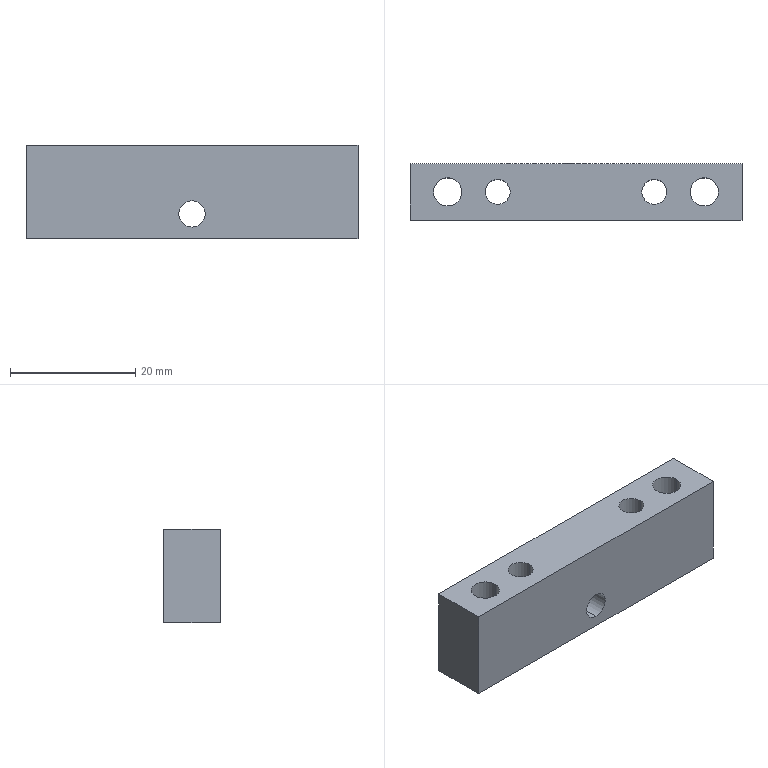Part | STEP file | 11-FG-B02411 | 1 solid | 22 faces | box 53 x 9 x 15 mm | volume 5874 mm3 | cylinder 14 | plane 8 | commonest cylinder face diameters 4 x4 4.5 x4 8 x4 4.2 x2
STEP:
#1=CARTESIAN_POINT('',(41.,4.5,15.));
#2=VERTEX_POINT('',#1);
#3=CARTESIAN_POINT('',(37.,4.5,15.));
#4=VERTEX_POINT('',#3);
#5=CARTESIAN_POINT('',(39.,4.5,15.));
#6=DIRECTION('',(0.,0.,-1.));
#7=DIRECTION('',(-1.,0.,0.));
#8=AXIS2_PLACEMENT_3D('',#5,#6,#7);
#9=CIRCLE('',#8,2.);
#10=EDGE_CURVE('',#2,#4,#9,.T.);
#11=ORIENTED_EDGE('',*,*,#10,.F.);
#12=CARTESIAN_POINT('',(41.,4.5,0.));
#13=VERTEX_POINT('',#12);
#14=CARTESIAN_POINT('',(41.,4.5,0.));
#15=DIRECTION('',(0.,0.,-1.));
#16=VECTOR('',#15,1000.);
#17=LINE('',#14,#16);
#18=EDGE_CURVE('',#2,#13,#17,.T.);
#19=ORIENTED_EDGE('',*,*,#18,.T.);
#20=CARTESIAN_POINT('',(37.,4.5,0.));
#21=VERTEX_POINT('',#20);
#22=CARTESIAN_POINT('',(39.,4.5,0.));
#23=DIRECTION('',(0.,0.,-1.));
#24=DIRECTION('',(-1.,0.,0.));
#25=AXIS2_PLACEMENT_3D('',#22,#23,#24);
#26=CIRCLE('',#25,2.);
#27=EDGE_CURVE('',#13,#21,#26,.T.);
#28=ORIENTED_EDGE('',*,*,#27,.T.);
#29=CARTESIAN_POINT('',(37.,4.5,0.));
#30=DIRECTION('',(0.,0.,-1.));
#31=VECTOR('',#30,1000.);
#32=LINE('',#29,#31);
#33=EDGE_CURVE('',#4,#21,#32,.T.);
#34=ORIENTED_EDGE('',*,*,#33,.F.);
#35=EDGE_LOOP('',(#11,#19,#28,#34));
#36=FACE_OUTER_BOUND('',#35,.T.);
#37=CARTESIAN_POINT('',(39.,4.5,0.));
#38=DIRECTION('',(0.,0.,-1.));
#39=DIRECTION('',(-1.,0.,0.));
#40=AXIS2_PLACEMENT_3D('',#37,#38,#39);
#41=CYLINDRICAL_SURFACE('',#40,2.);
#42=ADVANCED_FACE('',(#36),#41,.F.);
#43=CARTESIAN_POINT('',(16.,4.5,15.));
#44=VERTEX_POINT('',#43);
#45=CARTESIAN_POINT('',(12.,4.5,15.));
#46=VERTEX_POINT('',#45);
#47=CARTESIAN_POINT('',(14.,4.5,15.));
#48=DIRECTION('',(0.,0.,-1.));
#49=DIRECTION('',(-1.,0.,0.));
#50=AXIS2_PLACEMENT_3D('',#47,#48,#49);
#51=CIRCLE('',#50,2.);
#52=EDGE_CURVE('',#44,#46,#51,.T.);
#53=ORIENTED_EDGE('',*,*,#52,.F.);
#54=CARTESIAN_POINT('',(16.,4.5,0.));
#55=VERTEX_POINT('',#54);
#56=CARTESIAN_POINT('',(16.,4.5,0.));
#57=DIRECTION('',(0.,0.,-1.));
#58=VECTOR('',#57,1000.);
#59=LINE('',#56,#58);
#60=EDGE_CURVE('',#44,#55,#59,.T.);
#61=ORIENTED_EDGE('',*,*,#60,.T.);
#62=CARTESIAN_POINT('',(12.,4.5,0.));
#63=VERTEX_POINT('',#62);
#64=CARTESIAN_POINT('',(14.,4.5,0.));
#65=DIRECTION('',(0.,0.,-1.));
#66=DIRECTION('',(-1.,0.,0.));
#67=AXIS2_PLACEMENT_3D('',#64,#65,#66);
#68=CIRCLE('',#67,2.);
#69=EDGE_CURVE('',#55,#63,#68,.T.);
#70=ORIENTED_EDGE('',*,*,#69,.T.);
#71=CARTESIAN_POINT('',(12.,4.5,0.));
#72=DIRECTION('',(0.,0.,-1.));
#73=VECTOR('',#72,1000.);
#74=LINE('',#71,#73);
#75=EDGE_CURVE('',#46,#63,#74,.T.);
#76=ORIENTED_EDGE('',*,*,#75,.F.);
#77=EDGE_LOOP('',(#53,#61,#70,#76));
#78=FACE_OUTER_BOUND('',#77,.T.);
#79=CARTESIAN_POINT('',(14.,4.5,0.));
#80=DIRECTION('',(0.,0.,-1.));
#81=DIRECTION('',(-1.,0.,0.));
#82=AXIS2_PLACEMENT_3D('',#79,#80,#81);
#83=CYLINDRICAL_SURFACE('',#82,2.);
#84=ADVANCED_FACE('',(#78),#83,.F.);
#85=CARTESIAN_POINT('',(26.5,0.,1.9));
#86=VERTEX_POINT('',#85);
#87=CARTESIAN_POINT('',(26.5,0.,6.1));
#88=VERTEX_POINT('',#87);
#89=CARTESIAN_POINT('',(26.5,0.,4.));
#90=DIRECTION('',(0.,1.,0.));
#91=DIRECTION('',(0.,0.,1.));
#92=AXIS2_PLACEMENT_3D('',#89,#90,#91);
#93=CIRCLE('',#92,2.1);
#94=EDGE_CURVE('',#86,#88,#93,.T.);
#95=ORIENTED_EDGE('',*,*,#94,.F.);
#96=CARTESIAN_POINT('',(26.5,9.,1.9));
#97=VERTEX_POINT('',#96);
#98=CARTESIAN_POINT('',(26.5,9.,1.9));
#99=DIRECTION('',(0.,1.,0.));
#100=VECTOR('',#99,1000.);
#101=LINE('',#98,#100);
#102=EDGE_CURVE('',#86,#97,#101,.T.);
#103=ORIENTED_EDGE('',*,*,#102,.T.);
#104=CARTESIAN_POINT('',(26.5,9.,6.1));
#105=VERTEX_POINT('',#104);
#106=CARTESIAN_POINT('',(26.5,9.,4.));
#107=DIRECTION('',(0.,1.,0.));
#108=DIRECTION('',(0.,0.,1.));
#109=AXIS2_PLACEMENT_3D('',#106,#107,#108);
#110=CIRCLE('',#109,2.1);
#111=EDGE_CURVE('',#97,#105,#110,.T.);
#112=ORIENTED_EDGE('',*,*,#111,.T.);
#113=CARTESIAN_POINT('',(26.5,9.,6.1));
#114=DIRECTION('',(0.,1.,0.));
#115=VECTOR('',#114,1000.);
#116=LINE('',#113,#115);
#117=EDGE_CURVE('',#88,#105,#116,.T.);
#118=ORIENTED_EDGE('',*,*,#117,.F.);
#119=EDGE_LOOP('',(#95,#103,#112,#118));
#120=FACE_OUTER_BOUND('',#119,.T.);
#121=CARTESIAN_POINT('',(26.5,9.,4.));
#122=DIRECTION('',(0.,1.,0.));
#123=DIRECTION('',(0.,0.,1.));
#124=AXIS2_PLACEMENT_3D('',#121,#122,#123);
#125=CYLINDRICAL_SURFACE('',#124,2.1);
#126=ADVANCED_FACE('',(#120),#125,.F.);
#127=CARTESIAN_POINT('',(51.,4.5,4.4));
#128=VERTEX_POINT('',#127);
#129=CARTESIAN_POINT('',(43.,4.5,4.4));
#130=VERTEX_POINT('',#129);
#131=CARTESIAN_POINT('',(47.,4.5,4.4));
#132=DIRECTION('',(0.,0.,-1.));
#133=DIRECTION('',(-1.,0.,0.));
#134=AXIS2_PLACEMENT_3D('',#131,#132,#133);
#135=CIRCLE('',#134,4.);
#136=EDGE_CURVE('',#128,#130,#135,.T.);
#137=ORIENTED_EDGE('',*,*,#136,.F.);
#138=CARTESIAN_POINT('',(51.,4.5,0.));
#139=VERTEX_POINT('',#138);
#140=CARTESIAN_POINT('',(51.,4.5,0.));
#141=DIRECTION('',(0.,0.,-1.));
#142=VECTOR('',#141,1000.);
#143=LINE('',#140,#142);
#144=EDGE_CURVE('',#128,#139,#143,.T.);
#145=ORIENTED_EDGE('',*,*,#144,.T.);
#146=CARTESIAN_POINT('',(43.,4.5,0.));
#147=VERTEX_POINT('',#146);
#148=CARTESIAN_POINT('',(47.,4.5,0.));
#149=DIRECTION('',(0.,0.,-1.));
#150=DIRECTION('',(-1.,0.,0.));
#151=AXIS2_PLACEMENT_3D('',#148,#149,#150);
#152=CIRCLE('',#151,4.);
#153=EDGE_CURVE('',#139,#147,#152,.T.);
#154=ORIENTED_EDGE('',*,*,#153,.T.);
#155=CARTESIAN_POINT('',(43.,4.5,0.));
#156=DIRECTION('',(0.,0.,-1.));
#157=VECTOR('',#156,1000.);
#158=LINE('',#155,#157);
#159=EDGE_CURVE('',#130,#147,#158,.T.);
#160=ORIENTED_EDGE('',*,*,#159,.F.);
#161=EDGE_LOOP('',(#137,#145,#154,#160));
#162=FACE_OUTER_BOUND('',#161,.T.);
#163=CARTESIAN_POINT('',(47.,4.5,0.));
#164=DIRECTION('',(0.,0.,-1.));
#165=DIRECTION('',(-1.,0.,0.));
#166=AXIS2_PLACEMENT_3D('',#163,#164,#165);
#167=CYLINDRICAL_SURFACE('',#166,4.);
#168=ADVANCED_FACE('',(#162),#167,.F.);
#169=CARTESIAN_POINT('',(49.25,4.5,15.));
#170=VERTEX_POINT('',#169);
#171=CARTESIAN_POINT('',(44.75,4.5,15.));
#172=VERTEX_POINT('',#171);
#173=CARTESIAN_POINT('',(47.,4.5,15.));
#174=DIRECTION('',(0.,0.,-1.));
#175=DIRECTION('',(-1.,0.,0.));
#176=AXIS2_PLACEMENT_3D('',#173,#174,#175);
#177=CIRCLE('',#176,2.25);
#178=EDGE_CURVE('',#170,#172,#177,.T.);
#179=ORIENTED_EDGE('',*,*,#178,.F.);
#180=CARTESIAN_POINT('',(49.25,4.5,4.4));
#181=VERTEX_POINT('',#180);
#182=CARTESIAN_POINT('',(49.25,4.5,0.));
#183=DIRECTION('',(0.,0.,-1.));
#184=VECTOR('',#183,1000.);
#185=LINE('',#182,#184);
#186=EDGE_CURVE('',#170,#181,#185,.T.);
#187=ORIENTED_EDGE('',*,*,#186,.T.);
#188=CARTESIAN_POINT('',(44.75,4.5,4.4));
#189=VERTEX_POINT('',#188);
#190=CARTESIAN_POINT('',(47.,4.5,4.4));
#191=DIRECTION('',(0.,0.,-1.));
#192=DIRECTION('',(-1.,0.,0.));
#193=AXIS2_PLACEMENT_3D('',#190,#191,#192);
#194=CIRCLE('',#193,2.25);
#195=EDGE_CURVE('',#181,#189,#194,.T.);
#196=ORIENTED_EDGE('',*,*,#195,.T.);
#197=CARTESIAN_POINT('',(44.75,4.5,0.));
#198=DIRECTION('',(0.,0.,-1.));
#199=VECTOR('',#198,1000.);
#200=LINE('',#197,#199);
#201=EDGE_CURVE('',#172,#189,#200,.T.);
#202=ORIENTED_EDGE('',*,*,#201,.F.);
#203=EDGE_LOOP('',(#179,#187,#196,#202));
#204=FACE_OUTER_BOUND('',#203,.T.);
#205=CARTESIAN_POINT('',(47.,4.5,0.));
#206=DIRECTION('',(0.,0.,-1.));
#207=DIRECTION('',(-1.,0.,0.));
#208=AXIS2_PLACEMENT_3D('',#205,#206,#207);
#209=CYLINDRICAL_SURFACE('',#208,2.25);
#210=ADVANCED_FACE('',(#204),#209,.F.);
#211=CARTESIAN_POINT('',(10.,4.5,4.4));
#212=VERTEX_POINT('',#211);
#213=CARTESIAN_POINT('',(2.,4.5,4.4));
#214=VERTEX_POINT('',#213);
#215=CARTESIAN_POINT('',(6.,4.5,4.4));
#216=DIRECTION('',(0.,0.,-1.));
#217=DIRECTION('',(-1.,0.,0.));
#218=AXIS2_PLACEMENT_3D('',#215,#216,#217);
#219=CIRCLE('',#218,4.);
#220=EDGE_CURVE('',#212,#214,#219,.T.);
#221=ORIENTED_EDGE('',*,*,#220,.F.);
#222=CARTESIAN_POINT('',(10.,4.5,0.));
#223=VERTEX_POINT('',#222);
#224=CARTESIAN_POINT('',(10.,4.5,0.));
#225=DIRECTION('',(0.,0.,-1.));
#226=VECTOR('',#225,1000.);
#227=LINE('',#224,#226);
#228=EDGE_CURVE('',#212,#223,#227,.T.);
#229=ORIENTED_EDGE('',*,*,#228,.T.);
#230=CARTESIAN_POINT('',(2.,4.5,0.));
#231=VERTEX_POINT('',#230);
#232=CARTESIAN_POINT('',(6.,4.5,0.));
#233=DIRECTION('',(0.,0.,-1.));
#234=DIRECTION('',(-1.,0.,0.));
#235=AXIS2_PLACEMENT_3D('',#232,#233,#234);
#236=CIRCLE('',#235,4.);
#237=EDGE_CURVE('',#223,#231,#236,.T.);
#238=ORIENTED_EDGE('',*,*,#237,.T.);
#239=CARTESIAN_POINT('',(2.,4.5,0.));
#240=DIRECTION('',(0.,0.,-1.));
#241=VECTOR('',#240,1000.);
#242=LINE('',#239,#241);
#243=EDGE_CURVE('',#214,#231,#242,.T.);
#244=ORIENTED_EDGE('',*,*,#243,.F.);
#245=EDGE_LOOP('',(#221,#229,#238,#244));
#246=FACE_OUTER_BOUND('',#245,.T.);
#247=CARTESIAN_POINT('',(6.,4.5,0.));
#248=DIRECTION('',(0.,0.,-1.));
#249=DIRECTION('',(-1.,0.,0.));
#250=AXIS2_PLACEMENT_3D('',#247,#248,#249);
#251=CYLINDRICAL_SURFACE('',#250,4.);
#252=ADVANCED_FACE('',(#246),#251,.F.);
#253=CARTESIAN_POINT('',(8.25,4.5,15.));
#254=VERTEX_POINT('',#253);
#255=CARTESIAN_POINT('',(3.75,4.5,15.));
#256=VERTEX_POINT('',#255);
#257=CARTESIAN_POINT('',(6.,4.5,15.));
#258=DIRECTION('',(0.,0.,-1.));
#259=DIRECTION('',(-1.,0.,0.));
#260=AXIS2_PLACEMENT_3D('',#257,#258,#259);
#261=CIRCLE('',#260,2.25);
#262=EDGE_CURVE('',#254,#256,#261,.T.);
#263=ORIENTED_EDGE('',*,*,#262,.F.);
#264=CARTESIAN_POINT('',(8.25,4.5,4.4));
#265=VERTEX_POINT('',#264);
#266=CARTESIAN_POINT('',(8.25,4.5,0.));
#267=DIRECTION('',(0.,0.,-1.));
#268=VECTOR('',#267,1000.);
#269=LINE('',#266,#268);
#270=EDGE_CURVE('',#254,#265,#269,.T.);
#271=ORIENTED_EDGE('',*,*,#270,.T.);
#272=CARTESIAN_POINT('',(3.75,4.5,4.4));
#273=VERTEX_POINT('',#272);
#274=CARTESIAN_POINT('',(6.,4.5,4.4));
#275=DIRECTION('',(0.,0.,-1.));
#276=DIRECTION('',(-1.,0.,0.));
#277=AXIS2_PLACEMENT_3D('',#274,#275,#276);
#278=CIRCLE('',#277,2.25);
#279=EDGE_CURVE('',#265,#273,#278,.T.);
#280=ORIENTED_EDGE('',*,*,#279,.T.);
#281=CARTESIAN_POINT('',(3.75,4.5,0.));
#282=DIRECTION('',(0.,0.,-1.));
#283=VECTOR('',#282,1000.);
#284=LINE('',#281,#283);
#285=EDGE_CURVE('',#256,#273,#284,.T.);
#286=ORIENTED_EDGE('',*,*,#285,.F.);
#287=EDGE_LOOP('',(#263,#271,#280,#286));
#288=FACE_OUTER_BOUND('',#287,.T.);
#289=CARTESIAN_POINT('',(6.,4.5,0.));
#290=DIRECTION('',(0.,0.,-1.));
#291=DIRECTION('',(-1.,0.,0.));
#292=AXIS2_PLACEMENT_3D('',#289,#290,#291);
#293=CYLINDRICAL_SURFACE('',#292,2.25);
#294=ADVANCED_FACE('',(#288),#293,.F.);
#295=CARTESIAN_POINT('',(0.,9.,0.));
#296=VERTEX_POINT('',#295);
#297=CARTESIAN_POINT('',(0.,0.,0.));
#298=VERTEX_POINT('',#297);
#299=CARTESIAN_POINT('',(0.,0.,0.));
#300=DIRECTION('',(0.,-1.,0.));
#301=VECTOR('',#300,1000.);
#302=LINE('',#299,#301);
#303=EDGE_CURVE('',#296,#298,#302,.T.);
#304=ORIENTED_EDGE('',*,*,#303,.T.);
#305=CARTESIAN_POINT('',(0.,0.,15.));
#306=VERTEX_POINT('',#305);
#307=CARTESIAN_POINT('',(0.,0.,15.));
#308=DIRECTION('',(0.,0.,-1.));
#309=VECTOR('',#308,1000.);
#310=LINE('',#307,#309);
#311=EDGE_CURVE('',#306,#298,#310,.T.);
#312=ORIENTED_EDGE('',*,*,#311,.F.);
#313=CARTESIAN_POINT('',(0.,9.,15.));
#314=VERTEX_POINT('',#313);
#315=CARTESIAN_POINT('',(0.,0.,15.));
#316=DIRECTION('',(0.,-1.,0.));
#317=VECTOR('',#316,1000.);
#318=LINE('',#315,#317);
#319=EDGE_CURVE('',#314,#306,#318,.T.);
#320=ORIENTED_EDGE('',*,*,#319,.F.);
#321=CARTESIAN_POINT('',(0.,9.,15.));
#322=DIRECTION('',(0.,0.,-1.));
#323=VECTOR('',#322,1000.);
#324=LINE('',#321,#323);
#325=EDGE_CURVE('',#314,#296,#324,.T.);
#326=ORIENTED_EDGE('',*,*,#325,.T.);
#327=EDGE_LOOP('',(#304,#312,#320,#326));
#328=FACE_OUTER_BOUND('',#327,.T.);
#329=CARTESIAN_POINT('',(0.,0.,15.));
#330=DIRECTION('',(1.,0.,0.));
#331=DIRECTION('',(0.,1.,0.));
#332=AXIS2_PLACEMENT_3D('',#329,#330,#331);
#333=PLANE('',#332);
#334=ADVANCED_FACE('',(#328),#333,.F.);
#335=CARTESIAN_POINT('',(26.5,0.,4.));
#336=DIRECTION('',(0.,1.,0.));
#337=DIRECTION('',(0.,0.,1.));
#338=AXIS2_PLACEMENT_3D('',#335,#336,#337);
#339=CIRCLE('',#338,2.1);
#340=EDGE_CURVE('',#88,#86,#339,.T.);
#341=ORIENTED_EDGE('',*,*,#340,.T.);
#342=ORIENTED_EDGE('',*,*,#94,.T.);
#343=EDGE_LOOP('',(#341,#342));
#344=FACE_BOUND('',#343,.T.);
#345=CARTESIAN_POINT('',(53.,0.,0.));
#346=VERTEX_POINT('',#345);
#347=CARTESIAN_POINT('',(0.,0.,0.));
#348=DIRECTION('',(1.,0.,0.));
#349=VECTOR('',#348,1000.);
#350=LINE('',#347,#349);
#351=EDGE_CURVE('',#298,#346,#350,.T.);
#352=ORIENTED_EDGE('',*,*,#351,.T.);
#353=CARTESIAN_POINT('',(53.,0.,15.));
#354=VERTEX_POINT('',#353);
#355=CARTESIAN_POINT('',(53.,0.,15.));
#356=DIRECTION('',(0.,0.,-1.));
#357=VECTOR('',#356,1000.);
#358=LINE('',#355,#357);
#359=EDGE_CURVE('',#354,#346,#358,.T.);
#360=ORIENTED_EDGE('',*,*,#359,.F.);
#361=CARTESIAN_POINT('',(0.,0.,15.));
#362=DIRECTION('',(1.,0.,0.));
#363=VECTOR('',#362,1000.);
#364=LINE('',#361,#363);
#365=EDGE_CURVE('',#306,#354,#364,.T.);
#366=ORIENTED_EDGE('',*,*,#365,.F.);
#367=ORIENTED_EDGE('',*,*,#311,.T.);
#368=EDGE_LOOP('',(#352,#360,#366,#367));
#369=FACE_OUTER_BOUND('',#368,.T.);
#370=CARTESIAN_POINT('',(0.,0.,15.));
#371=DIRECTION('',(0.,1.,0.));
#372=DIRECTION('',(0.,0.,1.));
#373=AXIS2_PLACEMENT_3D('',#370,#371,#372);
#374=PLANE('',#373);
#375=ADVANCED_FACE('',(#344,#369),#374,.F.);
#376=CARTESIAN_POINT('',(53.,9.,0.));
#377=VERTEX_POINT('',#376);
#378=CARTESIAN_POINT('',(53.,0.,0.));
#379=DIRECTION('',(0.,1.,0.));
#380=VECTOR('',#379,1000.);
#381=LINE('',#378,#380);
#382=EDGE_CURVE('',#346,#377,#381,.T.);
#383=ORIENTED_EDGE('',*,*,#382,.T.);
#384=CARTESIAN_POINT('',(53.,9.,15.));
#385=VERTEX_POINT('',#384);
#386=CARTESIAN_POINT('',(53.,9.,15.));
#387=DIRECTION('',(0.,0.,-1.));
#388=VECTOR('',#387,1000.);
#389=LINE('',#386,#388);
#390=EDGE_CURVE('',#385,#377,#389,.T.);
#391=ORIENTED_EDGE('',*,*,#390,.F.);
#392=CARTESIAN_POINT('',(53.,0.,15.));
#393=DIRECTION('',(0.,1.,0.));
#394=VECTOR('',#393,1000.);
#395=LINE('',#392,#394);
#396=EDGE_CURVE('',#354,#385,#395,.T.);
#397=ORIENTED_EDGE('',*,*,#396,.F.);
#398=ORIENTED_EDGE('',*,*,#359,.T.);
#399=EDGE_LOOP('',(#383,#391,#397,#398));
#400=FACE_OUTER_BOUND('',#399,.T.);
#401=CARTESIAN_POINT('',(53.,0.,15.));
#402=DIRECTION('',(-1.,0.,0.));
#403=DIRECTION('',(0.,-1.,0.));
#404=AXIS2_PLACEMENT_3D('',#401,#402,#403);
#405=PLANE('',#404);
#406=ADVANCED_FACE('',(#400),#405,.F.);
#407=CARTESIAN_POINT('',(26.5,9.,4.));
#408=DIRECTION('',(0.,1.,0.));
#409=DIRECTION('',(0.,0.,1.));
#410=AXIS2_PLACEMENT_3D('',#407,#408,#409);
#411=CIRCLE('',#410,2.1);
#412=EDGE_CURVE('',#105,#97,#411,.T.);
#413=ORIENTED_EDGE('',*,*,#412,.F.);
#414=ORIENTED_EDGE('',*,*,#111,.F.);
#415=EDGE_LOOP('',(#413,#414));
#416=FACE_BOUND('',#415,.T.);
#417=CARTESIAN_POINT('',(0.,9.,0.));
#418=DIRECTION('',(-1.,0.,0.));
#419=VECTOR('',#418,1000.);
#420=LINE('',#417,#419);
#421=EDGE_CURVE('',#377,#296,#420,.T.);
#422=ORIENTED_EDGE('',*,*,#421,.T.);
#423=ORIENTED_EDGE('',*,*,#325,.F.);
#424=CARTESIAN_POINT('',(0.,9.,15.));
#425=DIRECTION('',(-1.,0.,0.));
#426=VECTOR('',#425,1000.);
#427=LINE('',#424,#426);
#428=EDGE_CURVE('',#385,#314,#427,.T.);
#429=ORIENTED_EDGE('',*,*,#428,.F.);
#430=ORIENTED_EDGE('',*,*,#390,.T.);
#431=EDGE_LOOP('',(#422,#423,#429,#430));
#432=FACE_OUTER_BOUND('',#431,.T.);
#433=CARTESIAN_POINT('',(0.,9.,15.));
#434=DIRECTION('',(0.,-1.,0.));
#435=DIRECTION('',(0.,0.,-1.));
#436=AXIS2_PLACEMENT_3D('',#433,#434,#435);
#437=PLANE('',#436);
#438=ADVANCED_FACE('',(#416,#432),#437,.F.);
#439=CARTESIAN_POINT('',(39.,4.5,15.));
#440=DIRECTION('',(0.,0.,-1.));
#441=DIRECTION('',(-1.,0.,0.));
#442=AXIS2_PLACEMENT_3D('',#439,#440,#441);
#443=CIRCLE('',#442,2.);
#444=EDGE_CURVE('',#4,#2,#443,.T.);
#445=ORIENTED_EDGE('',*,*,#444,.T.);
#446=ORIENTED_EDGE('',*,*,#10,.T.);
#447=EDGE_LOOP('',(#445,#446));
#448=FACE_BOUND('',#447,.T.);
#449=CARTESIAN_POINT('',(14.,4.5,15.));
#450=DIRECTION('',(0.,0.,-1.));
#451=DIRECTION('',(-1.,0.,0.));
#452=AXIS2_PLACEMENT_3D('',#449,#450,#451);
#453=CIRCLE('',#452,2.);
#454=EDGE_CURVE('',#46,#44,#453,.T.);
#455=ORIENTED_EDGE('',*,*,#454,.T.);
#456=ORIENTED_EDGE('',*,*,#52,.T.);
#457=EDGE_LOOP('',(#455,#456));
#458=FACE_BOUND('',#457,.T.);
#459=CARTESIAN_POINT('',(47.,4.5,15.));
#460=DIRECTION('',(0.,0.,-1.));
#461=DIRECTION('',(-1.,0.,0.));
#462=AXIS2_PLACEMENT_3D('',#459,#460,#461);
#463=CIRCLE('',#462,2.25);
#464=EDGE_CURVE('',#172,#170,#463,.T.);
#465=ORIENTED_EDGE('',*,*,#464,.T.);
#466=ORIENTED_EDGE('',*,*,#178,.T.);
#467=EDGE_LOOP('',(#465,#466));
#468=FACE_BOUND('',#467,.T.);
#469=CARTESIAN_POINT('',(6.,4.5,15.));
#470=DIRECTION('',(0.,0.,-1.));
#471=DIRECTION('',(-1.,0.,0.));
#472=AXIS2_PLACEMENT_3D('',#469,#470,#471);
#473=CIRCLE('',#472,2.25);
#474=EDGE_CURVE('',#256,#254,#473,.T.);
#475=ORIENTED_EDGE('',*,*,#474,.T.);
#476=ORIENTED_EDGE('',*,*,#262,.T.);
#477=EDGE_LOOP('',(#475,#476));
#478=FACE_BOUND('',#477,.T.);
#479=ORIENTED_EDGE('',*,*,#319,.T.);
#480=ORIENTED_EDGE('',*,*,#365,.T.);
#481=ORIENTED_EDGE('',*,*,#396,.T.);
#482=ORIENTED_EDGE('',*,*,#428,.T.);
#483=EDGE_LOOP('',(#479,#480,#481,#482));
#484=FACE_OUTER_BOUND('',#483,.T.);
#485=CARTESIAN_POINT('',(0.,9.,15.));
#486=DIRECTION('',(0.,0.,-1.));
#487=DIRECTION('',(-1.,0.,0.));
#488=AXIS2_PLACEMENT_3D('',#485,#486,#487);
#489=PLANE('',#488);
#490=ADVANCED_FACE('',(#448,#458,#468,#478,#484),#489,.F.);
#491=CARTESIAN_POINT('',(39.,4.5,0.));
#492=DIRECTION('',(0.,0.,-1.));
#493=DIRECTION('',(-1.,0.,0.));
#494=AXIS2_PLACEMENT_3D('',#491,#492,#493);
#495=CIRCLE('',#494,2.);
#496=EDGE_CURVE('',#21,#13,#495,.T.);
#497=ORIENTED_EDGE('',*,*,#496,.F.);
#498=ORIENTED_EDGE('',*,*,#27,.F.);
#499=EDGE_LOOP('',(#497,#498));
#500=FACE_BOUND('',#499,.T.);
#501=CARTESIAN_POINT('',(14.,4.5,0.));
#502=DIRECTION('',(0.,0.,-1.));
#503=DIRECTION('',(-1.,0.,0.));
#504=AXIS2_PLACEMENT_3D('',#501,#502,#503);
#505=CIRCLE('',#504,2.);
#506=EDGE_CURVE('',#63,#55,#505,.T.);
#507=ORIENTED_EDGE('',*,*,#506,.F.);
#508=ORIENTED_EDGE('',*,*,#69,.F.);
#509=EDGE_LOOP('',(#507,#508));
#510=FACE_BOUND('',#509,.T.);
#511=CARTESIAN_POINT('',(47.,4.5,0.));
#512=DIRECTION('',(0.,0.,-1.));
#513=DIRECTION('',(-1.,0.,0.));
#514=AXIS2_PLACEMENT_3D('',#511,#512,#513);
#515=CIRCLE('',#514,4.);
#516=EDGE_CURVE('',#147,#139,#515,.T.);
#517=ORIENTED_EDGE('',*,*,#516,.F.);
#518=ORIENTED_EDGE('',*,*,#153,.F.);
#519=EDGE_LOOP('',(#517,#518));
#520=FACE_BOUND('',#519,.T.);
#521=CARTESIAN_POINT('',(6.,4.5,0.));
#522=DIRECTION('',(0.,0.,-1.));
#523=DIRECTION('',(-1.,0.,0.));
#524=AXIS2_PLACEMENT_3D('',#521,#522,#523);
#525=CIRCLE('',#524,4.);
#526=EDGE_CURVE('',#231,#223,#525,.T.);
#527=ORIENTED_EDGE('',*,*,#526,.F.);
#528=ORIENTED_EDGE('',*,*,#237,.F.);
#529=EDGE_LOOP('',(#527,#528));
#530=FACE_BOUND('',#529,.T.);
#531=ORIENTED_EDGE('',*,*,#303,.F.);
#532=ORIENTED_EDGE('',*,*,#421,.F.);
#533=ORIENTED_EDGE('',*,*,#382,.F.);
#534=ORIENTED_EDGE('',*,*,#351,.F.);
#535=EDGE_LOOP('',(#531,#532,#533,#534));
#536=FACE_OUTER_BOUND('',#535,.T.);
#537=CARTESIAN_POINT('',(0.,9.,0.));
#538=DIRECTION('',(0.,0.,-1.));
#539=DIRECTION('',(-1.,0.,0.));
#540=AXIS2_PLACEMENT_3D('',#537,#538,#539);
#541=PLANE('',#540);
#542=ADVANCED_FACE('',(#500,#510,#520,#530,#536),#541,.T.);
#543=ORIENTED_EDGE('',*,*,#270,.F.);
#544=ORIENTED_EDGE('',*,*,#474,.F.);
#545=ORIENTED_EDGE('',*,*,#285,.T.);
#546=CARTESIAN_POINT('',(6.,4.5,4.4));
#547=DIRECTION('',(0.,0.,-1.));
#548=DIRECTION('',(-1.,0.,0.));
#549=AXIS2_PLACEMENT_3D('',#546,#547,#548);
#550=CIRCLE('',#549,2.25);
#551=EDGE_CURVE('',#273,#265,#550,.T.);
#552=ORIENTED_EDGE('',*,*,#551,.T.);
#553=EDGE_LOOP('',(#543,#544,#545,#552));
#554=FACE_OUTER_BOUND('',#553,.T.);
#555=CARTESIAN_POINT('',(6.,4.5,0.));
#556=DIRECTION('',(0.,0.,-1.));
#557=DIRECTION('',(-1.,0.,0.));
#558=AXIS2_PLACEMENT_3D('',#555,#556,#557);
#559=CYLINDRICAL_SURFACE('',#558,2.25);
#560=ADVANCED_FACE('',(#554),#559,.F.);
#561=ORIENTED_EDGE('',*,*,#551,.F.);
#562=ORIENTED_EDGE('',*,*,#279,.F.);
#563=EDGE_LOOP('',(#561,#562));
#564=FACE_BOUND('',#563,.T.);
#565=CARTESIAN_POINT('',(6.,4.5,4.4));
#566=DIRECTION('',(0.,0.,-1.));
#567=DIRECTION('',(-1.,0.,0.));
#568=AXIS2_PLACEMENT_3D('',#565,#566,#567);
#569=CIRCLE('',#568,4.);
#570=EDGE_CURVE('',#214,#212,#569,.T.);
#571=ORIENTED_EDGE('',*,*,#570,.T.);
#572=ORIENTED_EDGE('',*,*,#220,.T.);
#573=EDGE_LOOP('',(#571,#572));
#574=FACE_OUTER_BOUND('',#573,.T.);
#575=CARTESIAN_POINT('',(8.25,4.5,4.4));
#576=DIRECTION('',(0.,0.,1.));
#577=DIRECTION('',(1.,0.,0.));
#578=AXIS2_PLACEMENT_3D('',#575,#576,#577);
#579=PLANE('',#578);
#580=ADVANCED_FACE('',(#564,#574),#579,.F.);
#581=ORIENTED_EDGE('',*,*,#228,.F.);
#582=ORIENTED_EDGE('',*,*,#570,.F.);
#583=ORIENTED_EDGE('',*,*,#243,.T.);
#584=ORIENTED_EDGE('',*,*,#526,.T.);
#585=EDGE_LOOP('',(#581,#582,#583,#584));
#586=FACE_OUTER_BOUND('',#585,.T.);
#587=CARTESIAN_POINT('',(6.,4.5,0.));
#588=DIRECTION('',(0.,0.,-1.));
#589=DIRECTION('',(-1.,0.,0.));
#590=AXIS2_PLACEMENT_3D('',#587,#588,#589);
#591=CYLINDRICAL_SURFACE('',#590,4.);
#592=ADVANCED_FACE('',(#586),#591,.F.);
#593=ORIENTED_EDGE('',*,*,#186,.F.);
#594=ORIENTED_EDGE('',*,*,#464,.F.);
#595=ORIENTED_EDGE('',*,*,#201,.T.);
#596=CARTESIAN_POINT('',(47.,4.5,4.4));
#597=DIRECTION('',(0.,0.,-1.));
#598=DIRECTION('',(-1.,0.,0.));
#599=AXIS2_PLACEMENT_3D('',#596,#597,#598);
#600=CIRCLE('',#599,2.25);
#601=EDGE_CURVE('',#189,#181,#600,.T.);
#602=ORIENTED_EDGE('',*,*,#601,.T.);
#603=EDGE_LOOP('',(#593,#594,#595,#602));
#604=FACE_OUTER_BOUND('',#603,.T.);
#605=CARTESIAN_POINT('',(47.,4.5,0.));
#606=DIRECTION('',(0.,0.,-1.));
#607=DIRECTION('',(-1.,0.,0.));
#608=AXIS2_PLACEMENT_3D('',#605,#606,#607);
#609=CYLINDRICAL_SURFACE('',#608,2.25);
#610=ADVANCED_FACE('',(#604),#609,.F.);
#611=ORIENTED_EDGE('',*,*,#601,.F.);
#612=ORIENTED_EDGE('',*,*,#195,.F.);
#613=EDGE_LOOP('',(#611,#612));
#614=FACE_BOUND('',#613,.T.);
#615=CARTESIAN_POINT('',(47.,4.5,4.4));
#616=DIRECTION('',(0.,0.,-1.));
#617=DIRECTION('',(-1.,0.,0.));
#618=AXIS2_PLACEMENT_3D('',#615,#616,#617);
#619=CIRCLE('',#618,4.);
#620=EDGE_CURVE('',#130,#128,#619,.T.);
#621=ORIENTED_EDGE('',*,*,#620,.T.);
#622=ORIENTED_EDGE('',*,*,#136,.T.);
#623=EDGE_LOOP('',(#621,#622));
#624=FACE_OUTER_BOUND('',#623,.T.);
#625=CARTESIAN_POINT('',(49.25,4.5,4.4));
#626=DIRECTION('',(0.,0.,1.));
#627=DIRECTION('',(1.,0.,0.));
#628=AXIS2_PLACEMENT_3D('',#625,#626,#627);
#629=PLANE('',#628);
#630=ADVANCED_FACE('',(#614,#624),#629,.F.);
#631=ORIENTED_EDGE('',*,*,#144,.F.);
#632=ORIENTED_EDGE('',*,*,#620,.F.);
#633=ORIENTED_EDGE('',*,*,#159,.T.);
#634=ORIENTED_EDGE('',*,*,#516,.T.);
#635=EDGE_LOOP('',(#631,#632,#633,#634));
#636=FACE_OUTER_BOUND('',#635,.T.);
#637=CARTESIAN_POINT('',(47.,4.5,0.));
#638=DIRECTION('',(0.,0.,-1.));
#639=DIRECTION('',(-1.,0.,0.));
#640=AXIS2_PLACEMENT_3D('',#637,#638,#639);
#641=CYLINDRICAL_SURFACE('',#640,4.);
#642=ADVANCED_FACE('',(#636),#641,.F.);
#643=ORIENTED_EDGE('',*,*,#102,.F.);
#644=ORIENTED_EDGE('',*,*,#340,.F.);
#645=ORIENTED_EDGE('',*,*,#117,.T.);
#646=ORIENTED_EDGE('',*,*,#412,.T.);
#647=EDGE_LOOP('',(#643,#644,#645,#646));
#648=FACE_OUTER_BOUND('',#647,.T.);
#649=CARTESIAN_POINT('',(26.5,9.,4.));
#650=DIRECTION('',(0.,1.,0.));
#651=DIRECTION('',(0.,0.,1.));
#652=AXIS2_PLACEMENT_3D('',#649,#650,#651);
#653=CYLINDRICAL_SURFACE('',#652,2.1);
#654=ADVANCED_FACE('',(#648),#653,.F.);
#655=ORIENTED_EDGE('',*,*,#60,.F.);
#656=ORIENTED_EDGE('',*,*,#454,.F.);
#657=ORIENTED_EDGE('',*,*,#75,.T.);
#658=ORIENTED_EDGE('',*,*,#506,.T.);
#659=EDGE_LOOP('',(#655,#656,#657,#658));
#660=FACE_OUTER_BOUND('',#659,.T.);
#661=CARTESIAN_POINT('',(14.,4.5,0.));
#662=DIRECTION('',(0.,0.,-1.));
#663=DIRECTION('',(-1.,0.,0.));
#664=AXIS2_PLACEMENT_3D('',#661,#662,#663);
#665=CYLINDRICAL_SURFACE('',#664,2.);
#666=ADVANCED_FACE('',(#660),#665,.F.);
#667=ORIENTED_EDGE('',*,*,#18,.F.);
#668=ORIENTED_EDGE('',*,*,#444,.F.);
#669=ORIENTED_EDGE('',*,*,#33,.T.);
#670=ORIENTED_EDGE('',*,*,#496,.T.);
#671=EDGE_LOOP('',(#667,#668,#669,#670));
#672=FACE_OUTER_BOUND('',#671,.T.);
#673=CARTESIAN_POINT('',(39.,4.5,0.));
#674=DIRECTION('',(0.,0.,-1.));
#675=DIRECTION('',(-1.,0.,0.));
#676=AXIS2_PLACEMENT_3D('',#673,#674,#675);
#677=CYLINDRICAL_SURFACE('',#676,2.);
#678=ADVANCED_FACE('',(#672),#677,.F.);
#679=CLOSED_SHELL('',(#42,#84,#126,#168,#210,#252,#294,#334,#375,#406,#438,#490,#542,#560,#580,#592,#610,#630,#642,#654,#666,#678));
#680=MANIFOLD_SOLID_BREP('',#679);
#681=CARTESIAN_POINT('',(0.,0.,0.));
#682=DIRECTION('',(0.,0.,1.));
#683=DIRECTION('',(1.,0.,0.));
#684=AXIS2_PLACEMENT_3D('',#681,#682,#683);
#685=(LENGTH_UNIT()NAMED_UNIT(*)SI_UNIT(.MILLI.,.METRE.));
#686=UNCERTAINTY_MEASURE_WITH_UNIT(LENGTH_MEASURE(0.00001),#685,'','');
#687=(NAMED_UNIT(*)PLANE_ANGLE_UNIT()SI_UNIT($,.RADIAN.));
#688=(NAMED_UNIT(*)SI_UNIT($,.STERADIAN.)SOLID_ANGLE_UNIT());
#689=(GEOMETRIC_REPRESENTATION_CONTEXT(3)GLOBAL_UNCERTAINTY_ASSIGNED_CONTEXT((#686))GLOBAL_UNIT_ASSIGNED_CONTEXT((#685,#687,#688))REPRESENTATION_CONTEXT('',''));
#690=ADVANCED_BREP_SHAPE_REPRESENTATION('',(#680,#684),#689);